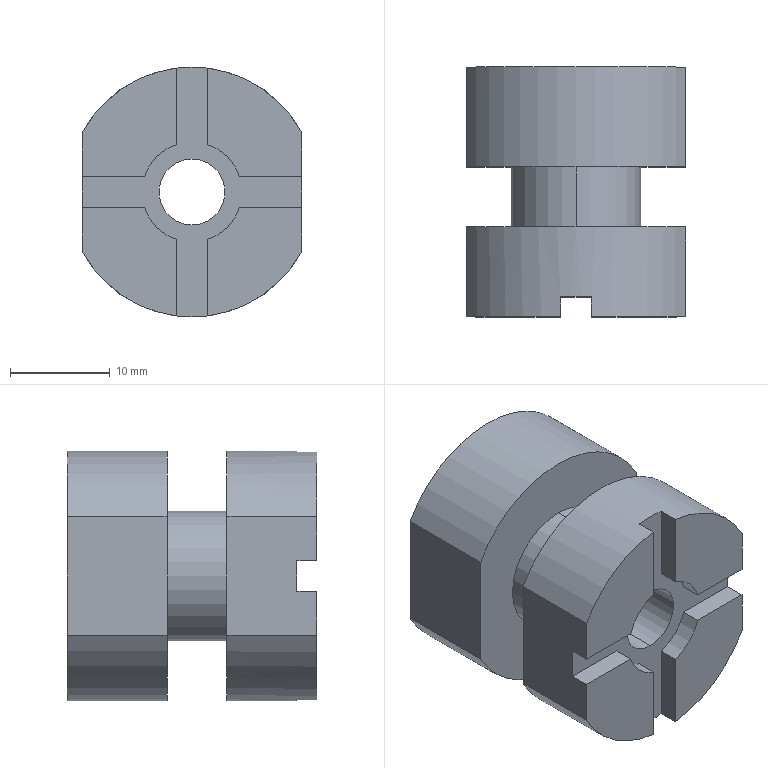Part | STEP file | push rod union | 1 solid | 37 faces | box 22 x 25 x 25 mm | volume 8188 mm3 | plane 21 | cylinder 16 | commonest cylinder face diameters 25 x6 10 x4 6.6 x2 11 x2 13 x2